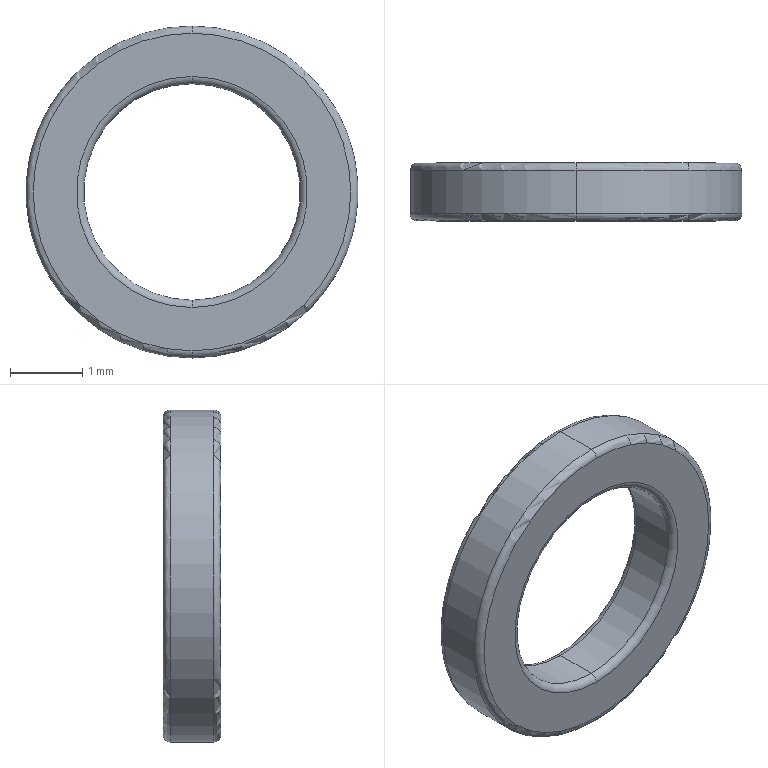Part | SolidWorks | features Extrusion 1, Fillet 1 | 1 solid | 14 faces | box 4.6 x 0.8 x 4.6 mm | volume 7.538 mm3 | torus 8 | cylinder 4 | plane 2 | commonest cylinder face diameters 3 x2 4.6 x2
STEP:
#1=CARTESIAN_POINT('',(0.,0.7,-2.3));
#2=VERTEX_POINT('',#1);
#3=CARTESIAN_POINT('',(0.,0.7,2.3));
#4=VERTEX_POINT('',#3);
#5=CARTESIAN_POINT('',(0.,0.7,0.));
#6=DIRECTION('',(0.,-1.,0.));
#7=DIRECTION('',(0.,0.,1.));
#8=AXIS2_PLACEMENT_3D('',#5,#6,#7);
#9=CIRCLE('',#8,2.3);
#10=EDGE_CURVE('',#2,#4,#9,.T.);
#11=ORIENTED_EDGE('',*,*,#10,.F.);
#12=CARTESIAN_POINT('',(0.,0.8,-2.2));
#13=VERTEX_POINT('',#12);
#14=CARTESIAN_POINT('',(0.,0.7,-2.2));
#15=DIRECTION('',(1.,0.,0.));
#16=DIRECTION('',(0.,0.,-1.));
#17=AXIS2_PLACEMENT_3D('',#14,#15,#16);
#18=CIRCLE('',#17,0.1);
#19=EDGE_CURVE('',#2,#13,#18,.T.);
#20=ORIENTED_EDGE('',*,*,#19,.T.);
#21=CARTESIAN_POINT('',(0.,0.8,2.2));
#22=VERTEX_POINT('',#21);
#23=CARTESIAN_POINT('',(0.,0.8,0.));
#24=DIRECTION('',(0.,1.,0.));
#25=DIRECTION('',(0.,0.,1.));
#26=AXIS2_PLACEMENT_3D('',#23,#24,#25);
#27=CIRCLE('',#26,2.2);
#28=EDGE_CURVE('',#22,#13,#27,.T.);
#29=ORIENTED_EDGE('',*,*,#28,.F.);
#30=CARTESIAN_POINT('',(0.,0.7,2.2));
#31=DIRECTION('',(-1.,0.,0.));
#32=DIRECTION('',(0.,0.,1.));
#33=AXIS2_PLACEMENT_3D('',#30,#31,#32);
#34=CIRCLE('',#33,0.1);
#35=EDGE_CURVE('',#4,#22,#34,.T.);
#36=ORIENTED_EDGE('',*,*,#35,.F.);
#37=EDGE_LOOP('',(#11,#20,#29,#36));
#38=FACE_OUTER_BOUND('',#37,.T.);
#39=CARTESIAN_POINT('',(0.,0.7,0.));
#40=DIRECTION('',(0.,1.,0.));
#41=DIRECTION('',(0.,0.,1.));
#42=AXIS2_PLACEMENT_3D('',#39,#40,#41);
#43=TOROIDAL_SURFACE('',#42,2.2,0.1);
#44=ADVANCED_FACE('',(#38),#43,.T.);
#45=CARTESIAN_POINT('',(0.,0.8,-1.6));
#46=VERTEX_POINT('',#45);
#47=CARTESIAN_POINT('',(0.,0.8,1.6));
#48=VERTEX_POINT('',#47);
#49=CARTESIAN_POINT('',(0.,0.8,0.));
#50=DIRECTION('',(0.,-1.,0.));
#51=DIRECTION('',(0.,0.,1.));
#52=AXIS2_PLACEMENT_3D('',#49,#50,#51);
#53=CIRCLE('',#52,1.6);
#54=EDGE_CURVE('',#46,#48,#53,.T.);
#55=ORIENTED_EDGE('',*,*,#54,.F.);
#56=CARTESIAN_POINT('',(0.,0.7,-1.5));
#57=VERTEX_POINT('',#56);
#58=CARTESIAN_POINT('',(0.,0.7,-1.6));
#59=DIRECTION('',(1.,0.,0.));
#60=DIRECTION('',(0.,0.,-1.));
#61=AXIS2_PLACEMENT_3D('',#58,#59,#60);
#62=CIRCLE('',#61,0.1);
#63=EDGE_CURVE('',#46,#57,#62,.T.);
#64=ORIENTED_EDGE('',*,*,#63,.T.);
#65=CARTESIAN_POINT('',(0.,0.7,1.5));
#66=VERTEX_POINT('',#65);
#67=CARTESIAN_POINT('',(0.,0.7,0.));
#68=DIRECTION('',(0.,1.,0.));
#69=DIRECTION('',(0.,0.,1.));
#70=AXIS2_PLACEMENT_3D('',#67,#68,#69);
#71=CIRCLE('',#70,1.5);
#72=EDGE_CURVE('',#66,#57,#71,.T.);
#73=ORIENTED_EDGE('',*,*,#72,.F.);
#74=CARTESIAN_POINT('',(0.,0.7,1.6));
#75=DIRECTION('',(-1.,0.,0.));
#76=DIRECTION('',(0.,0.,1.));
#77=AXIS2_PLACEMENT_3D('',#74,#75,#76);
#78=CIRCLE('',#77,0.1);
#79=EDGE_CURVE('',#48,#66,#78,.T.);
#80=ORIENTED_EDGE('',*,*,#79,.F.);
#81=EDGE_LOOP('',(#55,#64,#73,#80));
#82=FACE_OUTER_BOUND('',#81,.T.);
#83=CARTESIAN_POINT('',(0.,0.7,0.));
#84=DIRECTION('',(0.,1.,0.));
#85=DIRECTION('',(0.,0.,1.));
#86=AXIS2_PLACEMENT_3D('',#83,#84,#85);
#87=TOROIDAL_SURFACE('',#86,1.6,0.1);
#88=ADVANCED_FACE('',(#82),#87,.T.);
#89=CARTESIAN_POINT('',(0.,0.,-2.2));
#90=VERTEX_POINT('',#89);
#91=CARTESIAN_POINT('',(0.,0.,2.2));
#92=VERTEX_POINT('',#91);
#93=CARTESIAN_POINT('',(0.,0.,0.));
#94=DIRECTION('',(0.,-1.,0.));
#95=DIRECTION('',(0.,0.,1.));
#96=AXIS2_PLACEMENT_3D('',#93,#94,#95);
#97=CIRCLE('',#96,2.2);
#98=EDGE_CURVE('',#90,#92,#97,.T.);
#99=ORIENTED_EDGE('',*,*,#98,.F.);
#100=CARTESIAN_POINT('',(0.,0.1,-2.3));
#101=VERTEX_POINT('',#100);
#102=CARTESIAN_POINT('',(0.,0.1,-2.2));
#103=DIRECTION('',(1.,0.,0.));
#104=DIRECTION('',(0.,0.,-1.));
#105=AXIS2_PLACEMENT_3D('',#102,#103,#104);
#106=CIRCLE('',#105,0.1);
#107=EDGE_CURVE('',#90,#101,#106,.T.);
#108=ORIENTED_EDGE('',*,*,#107,.T.);
#109=CARTESIAN_POINT('',(0.,0.1,2.3));
#110=VERTEX_POINT('',#109);
#111=CARTESIAN_POINT('',(0.,0.1,0.));
#112=DIRECTION('',(0.,1.,0.));
#113=DIRECTION('',(0.,0.,1.));
#114=AXIS2_PLACEMENT_3D('',#111,#112,#113);
#115=CIRCLE('',#114,2.3);
#116=EDGE_CURVE('',#110,#101,#115,.T.);
#117=ORIENTED_EDGE('',*,*,#116,.F.);
#118=CARTESIAN_POINT('',(0.,0.1,2.2));
#119=DIRECTION('',(-1.,0.,0.));
#120=DIRECTION('',(0.,0.,1.));
#121=AXIS2_PLACEMENT_3D('',#118,#119,#120);
#122=CIRCLE('',#121,0.1);
#123=EDGE_CURVE('',#92,#110,#122,.T.);
#124=ORIENTED_EDGE('',*,*,#123,.F.);
#125=EDGE_LOOP('',(#99,#108,#117,#124));
#126=FACE_OUTER_BOUND('',#125,.T.);
#127=CARTESIAN_POINT('',(0.,0.1,0.));
#128=DIRECTION('',(0.,1.,0.));
#129=DIRECTION('',(0.,0.,1.));
#130=AXIS2_PLACEMENT_3D('',#127,#128,#129);
#131=TOROIDAL_SURFACE('',#130,2.2,0.1);
#132=ADVANCED_FACE('',(#126),#131,.T.);
#133=CARTESIAN_POINT('',(0.,0.1,-1.5));
#134=VERTEX_POINT('',#133);
#135=CARTESIAN_POINT('',(0.,0.1,1.5));
#136=VERTEX_POINT('',#135);
#137=CARTESIAN_POINT('',(0.,0.1,0.));
#138=DIRECTION('',(0.,-1.,0.));
#139=DIRECTION('',(0.,0.,1.));
#140=AXIS2_PLACEMENT_3D('',#137,#138,#139);
#141=CIRCLE('',#140,1.5);
#142=EDGE_CURVE('',#134,#136,#141,.T.);
#143=ORIENTED_EDGE('',*,*,#142,.F.);
#144=CARTESIAN_POINT('',(0.,0.,-1.6));
#145=VERTEX_POINT('',#144);
#146=CARTESIAN_POINT('',(0.,0.1,-1.6));
#147=DIRECTION('',(1.,0.,0.));
#148=DIRECTION('',(0.,0.,-1.));
#149=AXIS2_PLACEMENT_3D('',#146,#147,#148);
#150=CIRCLE('',#149,0.1);
#151=EDGE_CURVE('',#134,#145,#150,.T.);
#152=ORIENTED_EDGE('',*,*,#151,.T.);
#153=CARTESIAN_POINT('',(0.,0.,1.6));
#154=VERTEX_POINT('',#153);
#155=CARTESIAN_POINT('',(0.,0.,0.));
#156=DIRECTION('',(0.,1.,0.));
#157=DIRECTION('',(0.,0.,1.));
#158=AXIS2_PLACEMENT_3D('',#155,#156,#157);
#159=CIRCLE('',#158,1.6);
#160=EDGE_CURVE('',#154,#145,#159,.T.);
#161=ORIENTED_EDGE('',*,*,#160,.F.);
#162=CARTESIAN_POINT('',(0.,0.1,1.6));
#163=DIRECTION('',(-1.,0.,0.));
#164=DIRECTION('',(0.,0.,1.));
#165=AXIS2_PLACEMENT_3D('',#162,#163,#164);
#166=CIRCLE('',#165,0.1);
#167=EDGE_CURVE('',#136,#154,#166,.T.);
#168=ORIENTED_EDGE('',*,*,#167,.F.);
#169=EDGE_LOOP('',(#143,#152,#161,#168));
#170=FACE_OUTER_BOUND('',#169,.T.);
#171=CARTESIAN_POINT('',(0.,0.1,0.));
#172=DIRECTION('',(0.,1.,0.));
#173=DIRECTION('',(0.,0.,1.));
#174=AXIS2_PLACEMENT_3D('',#171,#172,#173);
#175=TOROIDAL_SURFACE('',#174,1.6,0.1);
#176=ADVANCED_FACE('',(#170),#175,.T.);
#177=CARTESIAN_POINT('',(0.,0.7,0.));
#178=DIRECTION('',(0.,1.,0.));
#179=DIRECTION('',(0.,0.,1.));
#180=AXIS2_PLACEMENT_3D('',#177,#178,#179);
#181=CIRCLE('',#180,1.5);
#182=EDGE_CURVE('',#57,#66,#181,.T.);
#183=ORIENTED_EDGE('',*,*,#182,.T.);
#184=CARTESIAN_POINT('',(0.,0.8,1.5));
#185=DIRECTION('',(0.,-1.,0.));
#186=VECTOR('',#185,1000.);
#187=LINE('',#184,#186);
#188=EDGE_CURVE('',#66,#136,#187,.T.);
#189=ORIENTED_EDGE('',*,*,#188,.T.);
#190=CARTESIAN_POINT('',(0.,0.1,0.));
#191=DIRECTION('',(0.,-1.,0.));
#192=DIRECTION('',(0.,0.,1.));
#193=AXIS2_PLACEMENT_3D('',#190,#191,#192);
#194=CIRCLE('',#193,1.5);
#195=EDGE_CURVE('',#136,#134,#194,.T.);
#196=ORIENTED_EDGE('',*,*,#195,.T.);
#197=CARTESIAN_POINT('',(0.,0.8,-1.5));
#198=DIRECTION('',(0.,-1.,0.));
#199=VECTOR('',#198,1000.);
#200=LINE('',#197,#199);
#201=EDGE_CURVE('',#57,#134,#200,.T.);
#202=ORIENTED_EDGE('',*,*,#201,.F.);
#203=EDGE_LOOP('',(#183,#189,#196,#202));
#204=FACE_OUTER_BOUND('',#203,.T.);
#205=CARTESIAN_POINT('',(0.,0.8,0.));
#206=DIRECTION('',(0.,-1.,0.));
#207=DIRECTION('',(0.,0.,-1.));
#208=AXIS2_PLACEMENT_3D('',#205,#206,#207);
#209=CYLINDRICAL_SURFACE('',#208,1.5);
#210=ADVANCED_FACE('',(#204),#209,.F.);
#211=ORIENTED_EDGE('',*,*,#10,.T.);
#212=CARTESIAN_POINT('',(0.,0.8,2.3));
#213=DIRECTION('',(0.,-1.,0.));
#214=VECTOR('',#213,1000.);
#215=LINE('',#212,#214);
#216=EDGE_CURVE('',#4,#110,#215,.T.);
#217=ORIENTED_EDGE('',*,*,#216,.T.);
#218=ORIENTED_EDGE('',*,*,#116,.T.);
#219=CARTESIAN_POINT('',(0.,0.8,-2.3));
#220=DIRECTION('',(0.,-1.,0.));
#221=VECTOR('',#220,1000.);
#222=LINE('',#219,#221);
#223=EDGE_CURVE('',#2,#101,#222,.T.);
#224=ORIENTED_EDGE('',*,*,#223,.F.);
#225=EDGE_LOOP('',(#211,#217,#218,#224));
#226=FACE_OUTER_BOUND('',#225,.T.);
#227=CARTESIAN_POINT('',(0.,0.8,0.));
#228=DIRECTION('',(0.,-1.,0.));
#229=DIRECTION('',(0.,0.,-1.));
#230=AXIS2_PLACEMENT_3D('',#227,#228,#229);
#231=CYLINDRICAL_SURFACE('',#230,2.3);
#232=ADVANCED_FACE('',(#226),#231,.T.);
#233=CARTESIAN_POINT('',(0.,0.8,0.));
#234=DIRECTION('',(0.,-1.,0.));
#235=DIRECTION('',(0.,0.,1.));
#236=AXIS2_PLACEMENT_3D('',#233,#234,#235);
#237=CIRCLE('',#236,1.6);
#238=EDGE_CURVE('',#48,#46,#237,.T.);
#239=ORIENTED_EDGE('',*,*,#238,.T.);
#240=ORIENTED_EDGE('',*,*,#54,.T.);
#241=EDGE_LOOP('',(#239,#240));
#242=FACE_BOUND('',#241,.T.);
#243=ORIENTED_EDGE('',*,*,#28,.T.);
#244=CARTESIAN_POINT('',(0.,0.8,0.));
#245=DIRECTION('',(0.,1.,0.));
#246=DIRECTION('',(0.,0.,1.));
#247=AXIS2_PLACEMENT_3D('',#244,#245,#246);
#248=CIRCLE('',#247,2.2);
#249=EDGE_CURVE('',#13,#22,#248,.T.);
#250=ORIENTED_EDGE('',*,*,#249,.T.);
#251=EDGE_LOOP('',(#243,#250));
#252=FACE_OUTER_BOUND('',#251,.T.);
#253=CARTESIAN_POINT('',(0.,0.8,0.));
#254=DIRECTION('',(0.,1.,0.));
#255=DIRECTION('',(0.,0.,1.));
#256=AXIS2_PLACEMENT_3D('',#253,#254,#255);
#257=PLANE('',#256);
#258=ADVANCED_FACE('',(#242,#252),#257,.T.);
#259=ORIENTED_EDGE('',*,*,#160,.T.);
#260=CARTESIAN_POINT('',(0.,0.,0.));
#261=DIRECTION('',(0.,1.,0.));
#262=DIRECTION('',(0.,0.,1.));
#263=AXIS2_PLACEMENT_3D('',#260,#261,#262);
#264=CIRCLE('',#263,1.6);
#265=EDGE_CURVE('',#145,#154,#264,.T.);
#266=ORIENTED_EDGE('',*,*,#265,.T.);
#267=EDGE_LOOP('',(#259,#266));
#268=FACE_BOUND('',#267,.T.);
#269=CARTESIAN_POINT('',(0.,0.,0.));
#270=DIRECTION('',(0.,-1.,0.));
#271=DIRECTION('',(0.,0.,1.));
#272=AXIS2_PLACEMENT_3D('',#269,#270,#271);
#273=CIRCLE('',#272,2.2);
#274=EDGE_CURVE('',#92,#90,#273,.T.);
#275=ORIENTED_EDGE('',*,*,#274,.T.);
#276=ORIENTED_EDGE('',*,*,#98,.T.);
#277=EDGE_LOOP('',(#275,#276));
#278=FACE_OUTER_BOUND('',#277,.T.);
#279=CARTESIAN_POINT('',(0.,0.,0.));
#280=DIRECTION('',(0.,1.,0.));
#281=DIRECTION('',(0.,0.,1.));
#282=AXIS2_PLACEMENT_3D('',#279,#280,#281);
#283=PLANE('',#282);
#284=ADVANCED_FACE('',(#268,#278),#283,.F.);
#285=ORIENTED_EDGE('',*,*,#216,.F.);
#286=CARTESIAN_POINT('',(0.,0.7,0.));
#287=DIRECTION('',(0.,-1.,0.));
#288=DIRECTION('',(0.,0.,1.));
#289=AXIS2_PLACEMENT_3D('',#286,#287,#288);
#290=CIRCLE('',#289,2.3);
#291=EDGE_CURVE('',#4,#2,#290,.T.);
#292=ORIENTED_EDGE('',*,*,#291,.T.);
#293=ORIENTED_EDGE('',*,*,#223,.T.);
#294=CARTESIAN_POINT('',(0.,0.1,0.));
#295=DIRECTION('',(0.,1.,0.));
#296=DIRECTION('',(0.,0.,1.));
#297=AXIS2_PLACEMENT_3D('',#294,#295,#296);
#298=CIRCLE('',#297,2.3);
#299=EDGE_CURVE('',#101,#110,#298,.T.);
#300=ORIENTED_EDGE('',*,*,#299,.T.);
#301=EDGE_LOOP('',(#285,#292,#293,#300));
#302=FACE_OUTER_BOUND('',#301,.T.);
#303=CARTESIAN_POINT('',(0.,0.8,0.));
#304=DIRECTION('',(0.,-1.,0.));
#305=DIRECTION('',(0.,0.,-1.));
#306=AXIS2_PLACEMENT_3D('',#303,#304,#305);
#307=CYLINDRICAL_SURFACE('',#306,2.3);
#308=ADVANCED_FACE('',(#302),#307,.T.);
#309=ORIENTED_EDGE('',*,*,#188,.F.);
#310=ORIENTED_EDGE('',*,*,#72,.T.);
#311=ORIENTED_EDGE('',*,*,#201,.T.);
#312=ORIENTED_EDGE('',*,*,#142,.T.);
#313=EDGE_LOOP('',(#309,#310,#311,#312));
#314=FACE_OUTER_BOUND('',#313,.T.);
#315=CARTESIAN_POINT('',(0.,0.8,0.));
#316=DIRECTION('',(0.,-1.,0.));
#317=DIRECTION('',(0.,0.,-1.));
#318=AXIS2_PLACEMENT_3D('',#315,#316,#317);
#319=CYLINDRICAL_SURFACE('',#318,1.5);
#320=ADVANCED_FACE('',(#314),#319,.F.);
#321=ORIENTED_EDGE('',*,*,#151,.F.);
#322=ORIENTED_EDGE('',*,*,#195,.F.);
#323=ORIENTED_EDGE('',*,*,#167,.T.);
#324=ORIENTED_EDGE('',*,*,#265,.F.);
#325=EDGE_LOOP('',(#321,#322,#323,#324));
#326=FACE_OUTER_BOUND('',#325,.T.);
#327=CARTESIAN_POINT('',(0.,0.1,0.));
#328=DIRECTION('',(0.,1.,0.));
#329=DIRECTION('',(0.,0.,1.));
#330=AXIS2_PLACEMENT_3D('',#327,#328,#329);
#331=TOROIDAL_SURFACE('',#330,1.6,0.1);
#332=ADVANCED_FACE('',(#326),#331,.T.);
#333=ORIENTED_EDGE('',*,*,#107,.F.);
#334=ORIENTED_EDGE('',*,*,#274,.F.);
#335=ORIENTED_EDGE('',*,*,#123,.T.);
#336=ORIENTED_EDGE('',*,*,#299,.F.);
#337=EDGE_LOOP('',(#333,#334,#335,#336));
#338=FACE_OUTER_BOUND('',#337,.T.);
#339=CARTESIAN_POINT('',(0.,0.1,0.));
#340=DIRECTION('',(0.,1.,0.));
#341=DIRECTION('',(0.,0.,1.));
#342=AXIS2_PLACEMENT_3D('',#339,#340,#341);
#343=TOROIDAL_SURFACE('',#342,2.2,0.1);
#344=ADVANCED_FACE('',(#338),#343,.T.);
#345=ORIENTED_EDGE('',*,*,#63,.F.);
#346=ORIENTED_EDGE('',*,*,#238,.F.);
#347=ORIENTED_EDGE('',*,*,#79,.T.);
#348=ORIENTED_EDGE('',*,*,#182,.F.);
#349=EDGE_LOOP('',(#345,#346,#347,#348));
#350=FACE_OUTER_BOUND('',#349,.T.);
#351=CARTESIAN_POINT('',(0.,0.7,0.));
#352=DIRECTION('',(0.,1.,0.));
#353=DIRECTION('',(0.,0.,1.));
#354=AXIS2_PLACEMENT_3D('',#351,#352,#353);
#355=TOROIDAL_SURFACE('',#354,1.6,0.1);
#356=ADVANCED_FACE('',(#350),#355,.T.);
#357=ORIENTED_EDGE('',*,*,#19,.F.);
#358=ORIENTED_EDGE('',*,*,#291,.F.);
#359=ORIENTED_EDGE('',*,*,#35,.T.);
#360=ORIENTED_EDGE('',*,*,#249,.F.);
#361=EDGE_LOOP('',(#357,#358,#359,#360));
#362=FACE_OUTER_BOUND('',#361,.T.);
#363=CARTESIAN_POINT('',(0.,0.7,0.));
#364=DIRECTION('',(0.,1.,0.));
#365=DIRECTION('',(0.,0.,1.));
#366=AXIS2_PLACEMENT_3D('',#363,#364,#365);
#367=TOROIDAL_SURFACE('',#366,2.2,0.1);
#368=ADVANCED_FACE('',(#362),#367,.T.);
#369=CLOSED_SHELL('',(#44,#88,#132,#176,#210,#232,#258,#284,#308,#320,#332,#344,#356,#368));
#370=MANIFOLD_SOLID_BREP('',#369);
#371=CARTESIAN_POINT('',(0.,0.,0.));
#372=DIRECTION('',(0.,0.,1.));
#373=DIRECTION('',(1.,0.,0.));
#374=AXIS2_PLACEMENT_3D('',#371,#372,#373);
#375=(LENGTH_UNIT()NAMED_UNIT(*)SI_UNIT(.MILLI.,.METRE.));
#376=UNCERTAINTY_MEASURE_WITH_UNIT(LENGTH_MEASURE(0.00001),#375,'','');
#377=(NAMED_UNIT(*)PLANE_ANGLE_UNIT()SI_UNIT($,.RADIAN.));
#378=(NAMED_UNIT(*)SI_UNIT($,.STERADIAN.)SOLID_ANGLE_UNIT());
#379=(GEOMETRIC_REPRESENTATION_CONTEXT(3)GLOBAL_UNCERTAINTY_ASSIGNED_CONTEXT((#376))GLOBAL_UNIT_ASSIGNED_CONTEXT((#375,#377,#378))REPRESENTATION_CONTEXT('',''));
#380=ADVANCED_BREP_SHAPE_REPRESENTATION('',(#370,#374),#379);